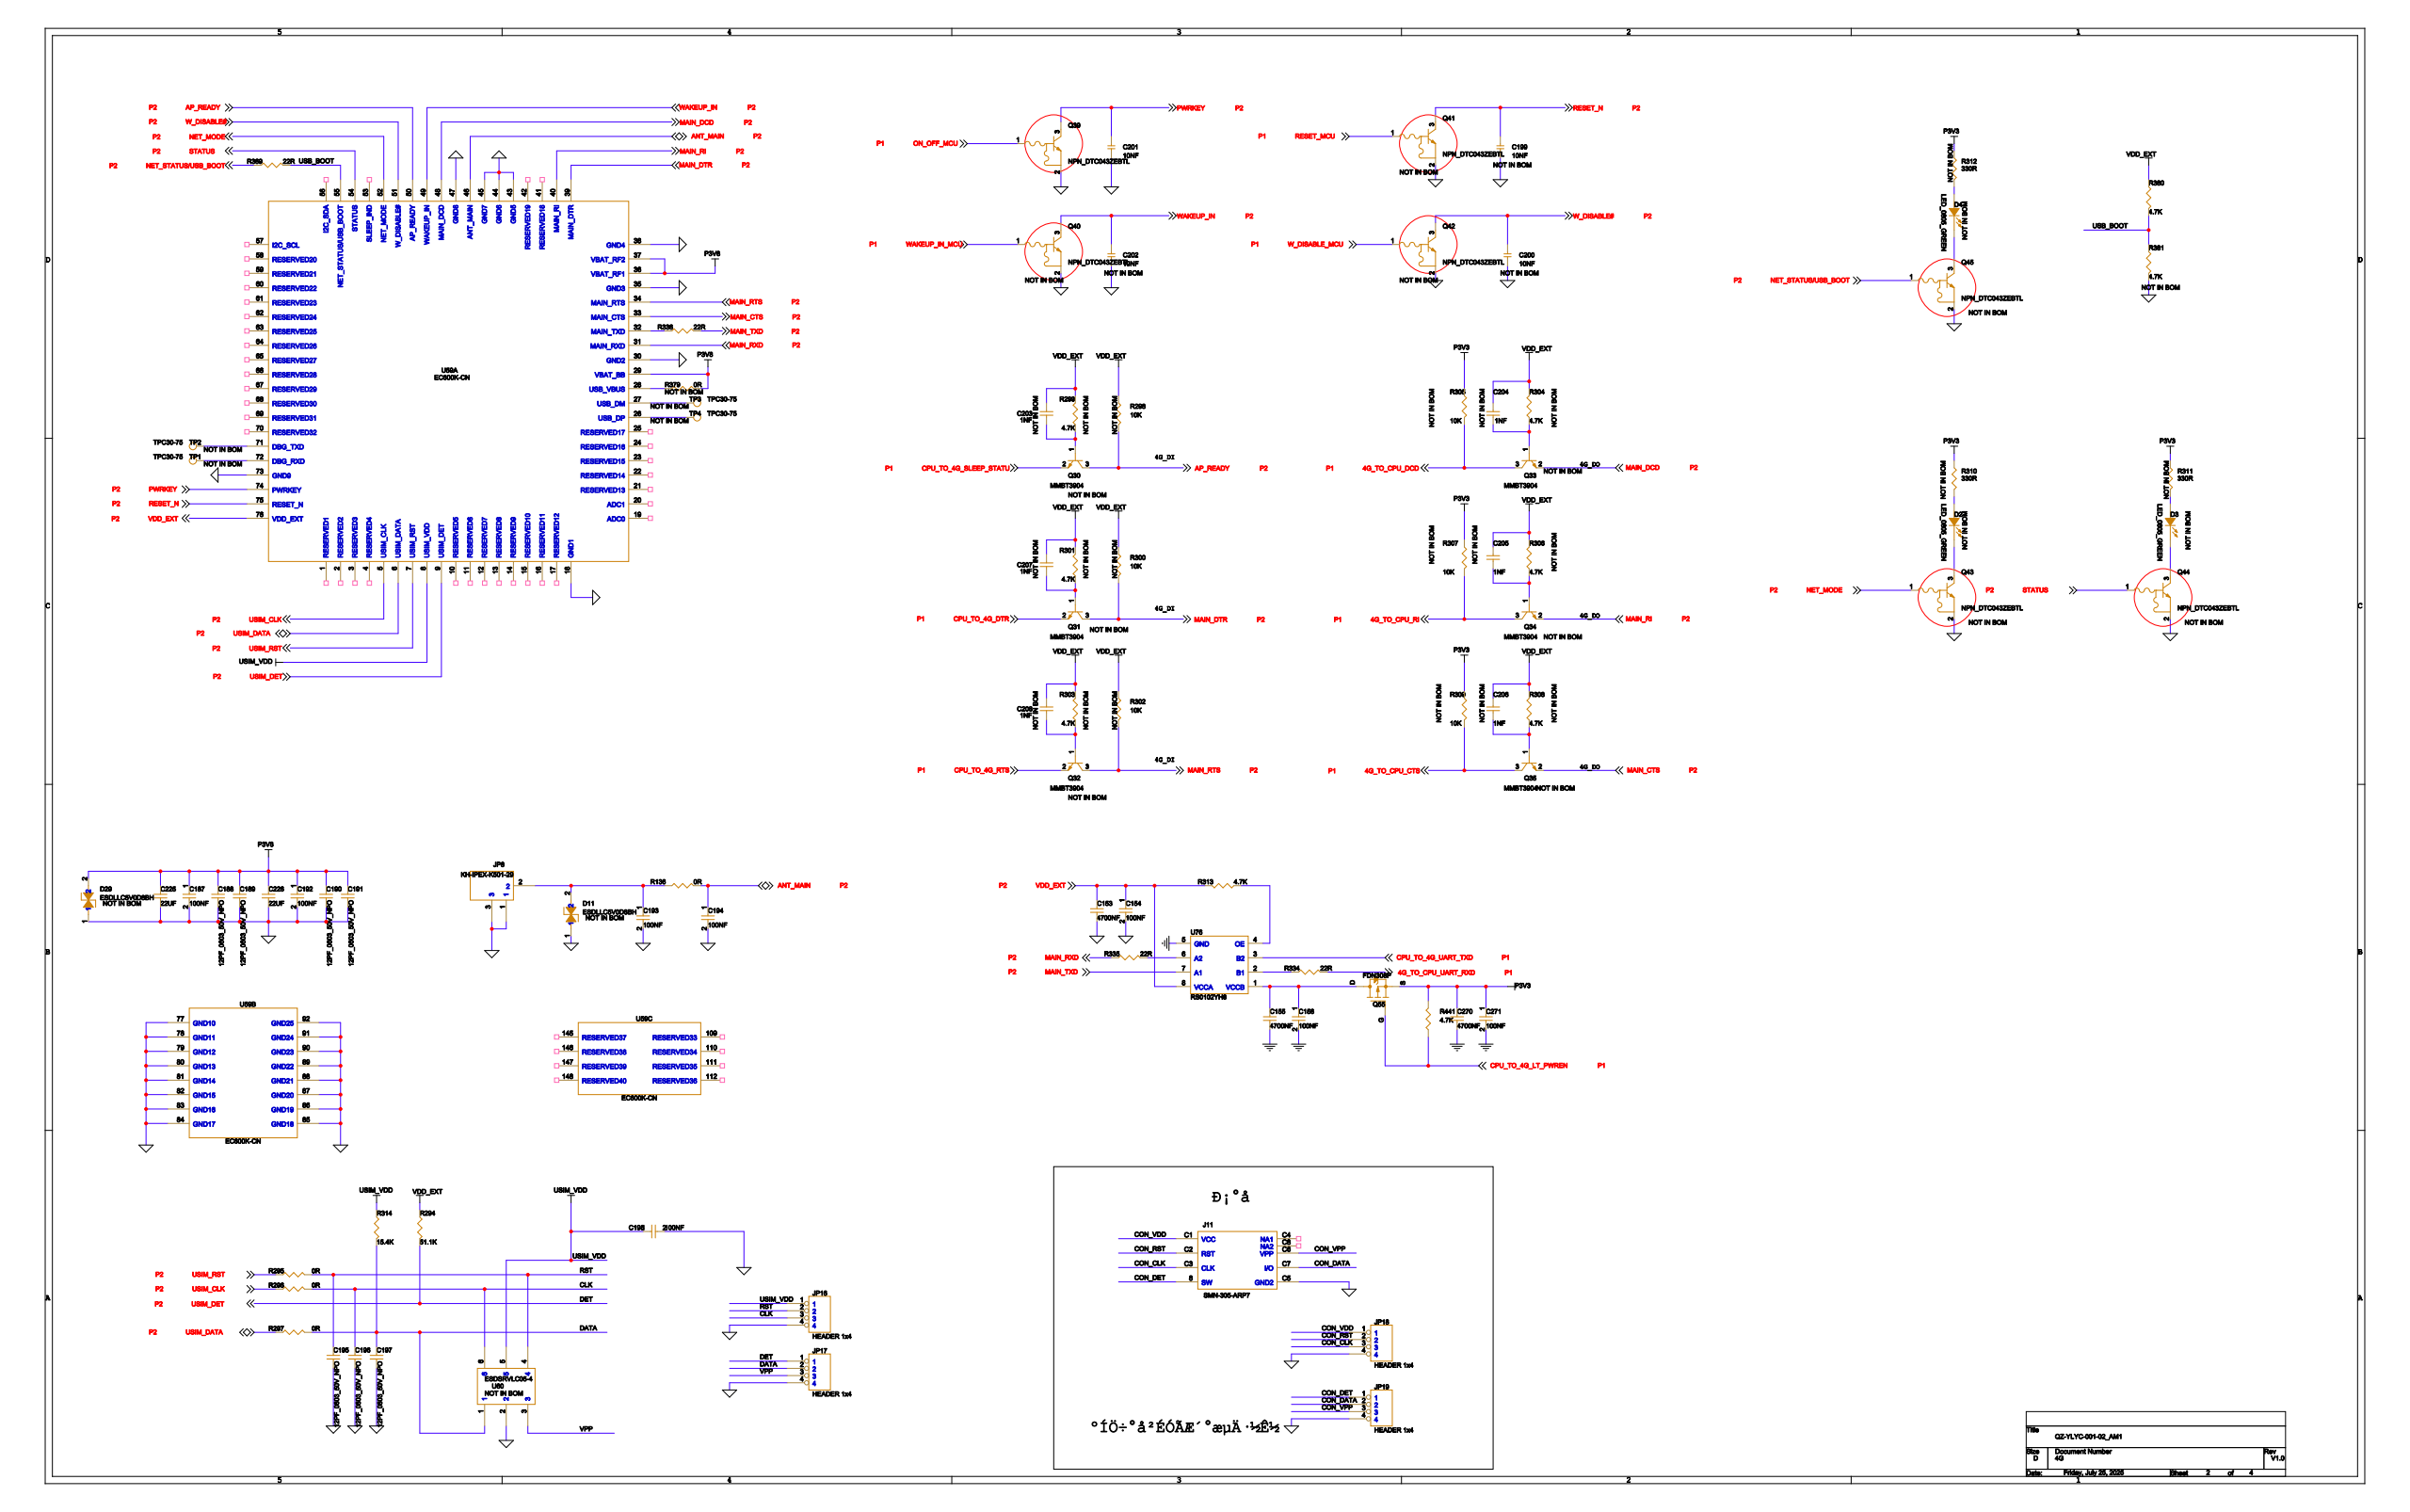Circuit board | Cadence Allegro | 366 parts | 230 nets | one sheet of the schematic
Parts on this sheet (reference | value | footprint):
C153 | C0603
C154 | C0603
C155 | C0603
C156 | C0603
C187 | C0603
C188 | C0603
C189 | C0603
C190 | C0603
C191 | C0603
C192 | C0603
C193 | C0603
C194 | C0603
C195 | C0603
C196 | C0603
C197 | C0603
C199 | C0603
C200 | C0603
C201 | C0603
C202 | C0603
C203 | C0603
C204 | C0603
C205 | C0603
C206 | C0603
C207 | C0603
C208 | C0603
C225 | C1206
C226 | C1206
C270 | C0603
C271 | C0603
D11 | DFN1006-2
D29 | DFN1006-2
J11 | MN-305-ARP7
JP8 | KH-IPEX-K501-29
JP16 | D1AX4N-2_54MM
JP17 | D1AX4N-2_54MM
JP18 | D1AX4N-2_54MM
JP19 | D1AX4N-2_54MM
Q30 | SOT23-123-095
Q31 | SOT23-123-095
Q32 | SOT23-123-095
Q33 | SOT23-123-095
Q34 | SOT23-123-095
Q35 | SOT23-123-095
Q39 | SOT_416FL
Q40 | SOT_416FL
Q41 | SOT_416FL
Q42 | SOT_416FL
Q43 | SOT_416FL
Q44 | SOT_416FL
Q45 | SOT_416FL
Q55 | SOT_23_IRLML6402
R136 | R0603
R294 | R0603
R295 | R0603
R296 | R0603
R297 | R0603
R298 | R0603
R299 | R0603
R300 | R0603
R301 | R0603
R302 | R0603
R303 | R0603
R304 | R0603
R305 | R0603
R306 | R0603
R307 | R0603
R308 | R0603
R309 | R0603
R310 | R0603
R311 | R0603
R312 | R0603
R313 | R0603
R314 | R0603
R334 | R0603
R335 | R0603
R336 | R0603
R369 | R0603
R379 | R1206
R380 | R0603
R381 | R0603
R441 | R0603
TP1 | TPC30-75
TP2 | TPC30-75
TP3 | TPC30-75
TP4 | TPC30-75
U59 | EC600K-CN
U60 | SOT23-6L
U76 | SOT23-8
Nets of these parts (net: part-pin ...):
USIM_VDD: JP16-1 R314-1 U60-5 U59-8
RST: C195-1 JP16-2 R295-2 U60-4
CLK: C196-1 JP16-3 R296-2 U60-6
GND_SIGNAL: C153-2 C154-2 C187-2 C188-2 C189-2 C190-2 C191-2 C192-2 C193-2 C194-2 C195-2 C196-2 C197-2 C199-1 C200-1 C201-1 C202-1 C225-2 C226-2 D11-1 D29-1 JP8-1 JP8-3 JP16-4 JP17-4 Q39-2 Q40-2 Q41-2 Q42-2 Q43-2 Q44-2 Q45-2 R381-2 U60-2 U59-18 U59-30 U59-35 U59-38 U59-43 U59-44 U59-45 U59-47 U59-73 U59-77 U59-78 U59-79 U59-80 U59-81 U59-82 U59-83 U59-84 U59-85 U59-86 U59-87 U59-88 U59-89 U59-90 U59-91 U59-92
USIM_DET: JP17-1 R294-2 U59-9
DATA: C197-1 JP17-2 R297-2 R314-2 U60-1
VPP: JP17-3 U60-3
CON_VDD: J11-C1 JP18-1
CON_RST: J11-C2 JP18-2
CON_CLK: J11-C3 JP18-3
CON_GND: J11-C5 JP18-4 JP19-4
CON_DET: J11-8 JP19-1
CON_DATA: J11-C7 JP19-2
CON_VPP: J11-C6 JP19-3
P3V8: C187-1 C188-1 C189-1 C190-1 C191-1 C192-1 C225-1 C226-1 D29-2 R379-2 U59-29 U59-36 U59-37
ON_OFF_MCU: Q39-1
PWRKEY: C201-2 Q39-3 U59-74
WAKEUP_IN_MCU: Q40-1
WAKEUP_IN: C202-2 Q40-3 U59-49
RESET_MCU: Q41-1
RESET_N: C199-2 Q41-3 U59-75
W_DISABLE_MCU: Q42-1
W_DISABLE#: C200-2 Q42-3 U59-51
NET_MODE: Q43-1 U59-52
N155134: Q43-3
STATUS: Q44-1 U59-54
N155598: Q44-3
NET_STATUS/USB_BOOT: Q45-1 R369-1
N155869: Q45-3
GND: C155-2 C156-2 C270-2 C271-2 U76-5
MAIN_TXD: R336-2 U76-7
N436365: R335-2 U76-6
N140708: R334-1 U76-2
CPU_TO_4G_UART_TXD: U76-3
N140470: R313-1 U76-4
VDD_EXT: C153-1 C154-1 C203-1 C204-1 C205-1 C206-1 C207-1 C208-1 R294-1 R298-1 R299-1 R300-1 R301-1 R302-1 R303-1 R304-1 R306-1 R308-1 R313-2 R380-1 U76-8 U59-76
N140728: C155-1 C156-1 Q55-D U76-1
P3V3: C270-1 C271-1 Q55-S R305-1 R307-1 R309-1 R310-1 R311-1 R312-1 R441-2
N140250: C193-1 D11-2 JP8-2 R136-1
ANT_MAIN: C194-1 R136-2 U59-46
N138922: C203-2 Q30-1 R299-2
N138918: C204-2 Q33-1 R304-2
N139304: C205-2 Q34-1 R306-2
N139744: C206-2 Q35-1 R308-2
N139344: C207-2 Q31-1 R301-2
N139760: C208-2 Q32-1 R303-2
N155435: R310-2
N155578: R311-2
N155849: R312-2
CPU_TO_4G_LT_PWREN: Q55-G R441-1
AP_READY: Q30-3 R298-2 U59-50
CPU_TO_4G_SLEEP_STATU: Q30-2
MAIN_DTR: Q31-3 R300-2 U59-39
CPU_TO_4G_DTR: Q31-2
MAIN_RTS: Q32-3 R302-2 U59-34
CPU_TO_4G_RTS: Q32-2
4G_TO_CPU_DCD: Q33-3 R305-2
MAIN_DCD: Q33-2 U59-48
4G_TO_CPU_RI: Q34-3 R307-2
MAIN_RI: Q34-2 U59-40
4G_TO_CPU_CTS: Q35-3 R309-2
MAIN_CTS: Q35-2 U59-33
N221468: R379-1 U59-28
USIM_RST: R295-1 U59-7
USIM_CLK: R296-1 U59-5
USIM_DATA: R297-1 U59-6
4G_TO_CPU_UART_RXD: R334-2
MAIN_RXD: R335-1 U59-31
N138710: R336-1 U59-32
USB_BOOT: R369-2 R380-2 R381-1 U59-55
N221299: TP1-1 U59-72
N221331: TP2-1 U59-71
N221391: TP3-1 U59-27
N221395: TP4-1 U59-26